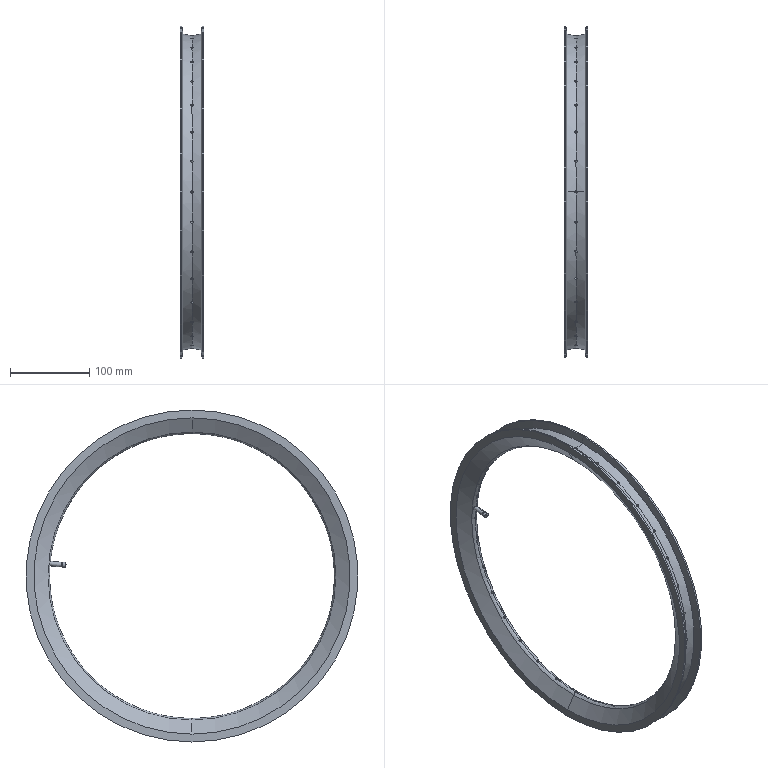Part | STEP file | KMX Rim | 1 solid | 98 faces | box 30 x 420 x 420 mm | volume 458838 mm3 | cylinder 74 | cone 14 | plane 6 | torus 4 | commonest cylinder face diameters 3 x64 420 x4 4.75 x2 6 x2 6.4 x2